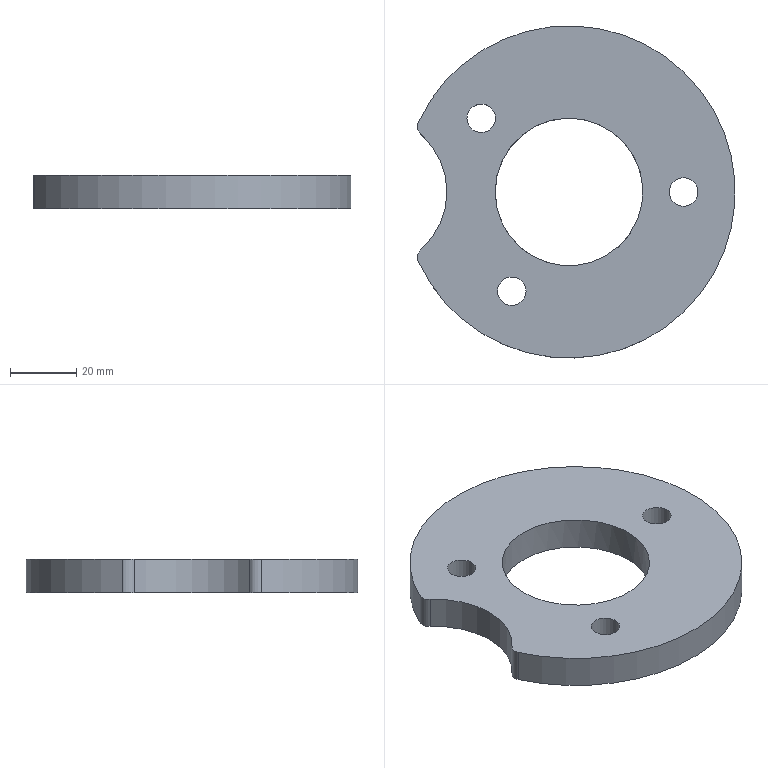Part | STEP file | 1_id1226_x_t | 1 solid | 10 faces | box 95.666 x 100 x 10 mm | volume 57810 mm3 | cylinder 8 | plane 2 | commonest cylinder face diameters 8.6 x3 6 x2 44.45 x1 46.5 x1 100 x1
STEP:
#1=CARTESIAN_POINT('',(0.,0.,0.));
#2=DIRECTION('',(0.,0.,1.));
#3=DIRECTION('',(1.,0.,0.));
#4=AXIS2_PLACEMENT_3D('',#1,#2,#3);
#5=CARTESIAN_POINT('',(817.535,308.471,90.11));
#6=VERTEX_POINT('',#5);
#7=CARTESIAN_POINT('',(817.535,266.529,90.11));
#8=VERTEX_POINT('',#7);
#9=CARTESIAN_POINT('',(862.925,287.5,90.11));
#10=DIRECTION('',(0.,0.,-1.));
#11=DIRECTION('',(1.,0.,0.));
#12=AXIS2_PLACEMENT_3D('',#9,#10,#11);
#13=CIRCLE('',#12,50.);
#14=CARTESIAN_POINT('',(862.925,287.5,90.11));
#15=DIRECTION('',(0.,0.,-1.));
#16=DIRECTION('',(-1.,0.,0.));
#17=AXIS2_PLACEMENT_3D('',#14,#15,#16);
#18=PLANE('',#17);
#19=CARTESIAN_POINT('',(0.,0.));
#20=DIRECTION('',(-1.,0.));
#21=AXIS2_PLACEMENT_2D('',#19,#20);
#22=CIRCLE('',#21,50.);
#23=(GEOMETRIC_REPRESENTATION_CONTEXT(2)PARAMETRIC_REPRESENTATION_CONTEXT()REPRESENTATION_CONTEXT('',''));
#24=DEFINITIONAL_REPRESENTATION('',(#22),#23);
#25=PCURVE('',#18,#24);
#26=CARTESIAN_POINT('',(862.925,287.5,100.11));
#27=DIRECTION('',(0.,0.,-1.));
#28=DIRECTION('',(-1.,0.,0.));
#29=AXIS2_PLACEMENT_3D('',#26,#27,#28);
#30=CYLINDRICAL_SURFACE('',#29,50.);
#31=CARTESIAN_POINT('',(-3.142,10.));
#32=DIRECTION('',(1.,0.));
#33=VECTOR('',#32,1.);
#34=LINE('',#31,#33);
#35=(GEOMETRIC_REPRESENTATION_CONTEXT(2)PARAMETRIC_REPRESENTATION_CONTEXT()REPRESENTATION_CONTEXT('',''));
#36=DEFINITIONAL_REPRESENTATION('',(#34),#35);
#37=PCURVE('',#30,#36);
#38=SURFACE_CURVE('',#13,(#25,#37),.PCURVE_S1.);
#39=EDGE_CURVE('',#6,#8,#38,.T.);
#40=ORIENTED_EDGE('',*,*,#39,.T.);
#41=CARTESIAN_POINT('',(818.278,270.04,90.11));
#42=VERTEX_POINT('',#41);
#43=CARTESIAN_POINT('',(820.259,267.787,90.11));
#44=DIRECTION('',(0.,0.,-1.));
#45=DIRECTION('',(-1.,0.,0.));
#46=AXIS2_PLACEMENT_3D('',#43,#44,#45);
#47=CIRCLE('',#46,3.);
#48=CARTESIAN_POINT('',(42.666,-19.713));
#49=DIRECTION('',(1.,0.));
#50=AXIS2_PLACEMENT_2D('',#48,#49);
#51=CIRCLE('',#50,3.);
#52=(GEOMETRIC_REPRESENTATION_CONTEXT(2)PARAMETRIC_REPRESENTATION_CONTEXT()REPRESENTATION_CONTEXT('',''));
#53=DEFINITIONAL_REPRESENTATION('',(#51),#52);
#54=PCURVE('',#18,#53);
#55=CARTESIAN_POINT('',(820.259,267.787,29.935));
#56=DIRECTION('',(0.,0.,1.));
#57=DIRECTION('',(1.,0.,0.));
#58=AXIS2_PLACEMENT_3D('',#55,#56,#57);
#59=CYLINDRICAL_SURFACE('',#58,3.);
#60=CARTESIAN_POINT('',(9.425,60.175));
#61=DIRECTION('',(-1.,0.));
#62=VECTOR('',#61,1.);
#63=LINE('',#60,#62);
#64=(GEOMETRIC_REPRESENTATION_CONTEXT(2)PARAMETRIC_REPRESENTATION_CONTEXT()REPRESENTATION_CONTEXT('',''));
#65=DEFINITIONAL_REPRESENTATION('',(#63),#64);
#66=PCURVE('',#59,#65);
#67=SURFACE_CURVE('',#47,(#54,#66),.PCURVE_S1.);
#68=EDGE_CURVE('',#8,#42,#67,.T.);
#69=ORIENTED_EDGE('',*,*,#68,.T.);
#70=CARTESIAN_POINT('',(818.278,304.96,90.11));
#71=VERTEX_POINT('',#70);
#72=CARTESIAN_POINT('',(802.925,287.5,90.11));
#73=DIRECTION('',(0.,0.,1.));
#74=DIRECTION('',(1.,0.,0.));
#75=AXIS2_PLACEMENT_3D('',#72,#73,#74);
#76=CIRCLE('',#75,23.25);
#77=CARTESIAN_POINT('',(36.75,0.));
#78=CARTESIAN_POINT('',(36.75,40.27));
#79=CARTESIAN_POINT('',(71.625,20.135));
#80=CARTESIAN_POINT('',(106.5,0.));
#81=CARTESIAN_POINT('',(71.625,-20.135));
#82=CARTESIAN_POINT('',(36.75,-40.27));
#83=CARTESIAN_POINT('',(36.75,0.));
#84=(BOUNDED_CURVE()B_SPLINE_CURVE(2,(#77,#78,#79,#80,#81,#82,#83),.UNSPECIFIED.,.T.,.F.)B_SPLINE_CURVE_WITH_KNOTS((1,2,2,2,2,1),(-2.094,0.,2.094,4.189,6.283,8.378),.UNSPECIFIED.)CURVE()GEOMETRIC_REPRESENTATION_ITEM()RATIONAL_B_SPLINE_CURVE((1.,0.5,1.,0.5,1.,0.5,1.))REPRESENTATION_ITEM(''));
#85=(GEOMETRIC_REPRESENTATION_CONTEXT(2)PARAMETRIC_REPRESENTATION_CONTEXT()REPRESENTATION_CONTEXT('',''));
#86=DEFINITIONAL_REPRESENTATION('',(#84),#85);
#87=PCURVE('',#18,#86);
#88=CARTESIAN_POINT('',(802.925,287.5,29.935));
#89=DIRECTION('',(0.,0.,1.));
#90=DIRECTION('',(1.,0.,0.));
#91=AXIS2_PLACEMENT_3D('',#88,#89,#90);
#92=CYLINDRICAL_SURFACE('',#91,23.25);
#93=CARTESIAN_POINT('',(0.,60.175));
#94=DIRECTION('',(1.,0.));
#95=VECTOR('',#94,1.);
#96=LINE('',#93,#95);
#97=(GEOMETRIC_REPRESENTATION_CONTEXT(2)PARAMETRIC_REPRESENTATION_CONTEXT()REPRESENTATION_CONTEXT('',''));
#98=DEFINITIONAL_REPRESENTATION('',(#96),#97);
#99=PCURVE('',#92,#98);
#100=SURFACE_CURVE('',#76,(#87,#99),.PCURVE_S1.);
#101=EDGE_CURVE('',#42,#71,#100,.T.);
#102=ORIENTED_EDGE('',*,*,#101,.T.);
#103=CARTESIAN_POINT('',(820.259,307.213,90.11));
#104=DIRECTION('',(0.,0.,-1.));
#105=DIRECTION('',(-1.,0.,0.));
#106=AXIS2_PLACEMENT_3D('',#103,#104,#105);
#107=CIRCLE('',#106,3.);
#108=CARTESIAN_POINT('',(42.666,19.713));
#109=DIRECTION('',(1.,0.));
#110=AXIS2_PLACEMENT_2D('',#108,#109);
#111=CIRCLE('',#110,3.);
#112=(GEOMETRIC_REPRESENTATION_CONTEXT(2)PARAMETRIC_REPRESENTATION_CONTEXT()REPRESENTATION_CONTEXT('',''));
#113=DEFINITIONAL_REPRESENTATION('',(#111),#112);
#114=PCURVE('',#18,#113);
#115=CARTESIAN_POINT('',(820.259,307.213,29.935));
#116=DIRECTION('',(0.,0.,-1.));
#117=DIRECTION('',(-1.,0.,0.));
#118=AXIS2_PLACEMENT_3D('',#115,#116,#117);
#119=CYLINDRICAL_SURFACE('',#118,3.);
#120=CARTESIAN_POINT('',(0.,-60.175));
#121=DIRECTION('',(1.,0.));
#122=VECTOR('',#121,1.);
#123=LINE('',#120,#122);
#124=(GEOMETRIC_REPRESENTATION_CONTEXT(2)PARAMETRIC_REPRESENTATION_CONTEXT()REPRESENTATION_CONTEXT('',''));
#125=DEFINITIONAL_REPRESENTATION('',(#123),#124);
#126=PCURVE('',#119,#125);
#127=SURFACE_CURVE('',#107,(#114,#126),.PCURVE_S1.);
#128=EDGE_CURVE('',#71,#6,#127,.T.);
#129=ORIENTED_EDGE('',*,*,#128,.T.);
#130=EDGE_LOOP('',(#40,#69,#102,#129));
#131=FACE_BOUND('',#130,.T.);
#132=CARTESIAN_POINT('',(840.7,287.5,90.11));
#133=VERTEX_POINT('',#132);
#134=CARTESIAN_POINT('',(862.925,287.5,90.11));
#135=DIRECTION('',(0.,0.,1.));
#136=DIRECTION('',(-1.,0.,0.));
#137=AXIS2_PLACEMENT_3D('',#134,#135,#136);
#138=CIRCLE('',#137,22.225);
#139=CARTESIAN_POINT('',(22.225,0.));
#140=CARTESIAN_POINT('',(22.225,-38.495));
#141=CARTESIAN_POINT('',(-11.113,-19.247));
#142=CARTESIAN_POINT('',(-44.45,0.));
#143=CARTESIAN_POINT('',(-11.113,19.247));
#144=CARTESIAN_POINT('',(22.225,38.495));
#145=CARTESIAN_POINT('',(22.225,0.));
#146=(BOUNDED_CURVE()B_SPLINE_CURVE(2,(#139,#140,#141,#142,#143,#144,#145),.UNSPECIFIED.,.T.,.F.)B_SPLINE_CURVE_WITH_KNOTS((1,2,2,2,2,1),(-2.094,0.,2.094,4.189,6.283,8.378),.UNSPECIFIED.)CURVE()GEOMETRIC_REPRESENTATION_ITEM()RATIONAL_B_SPLINE_CURVE((1.,0.5,1.,0.5,1.,0.5,1.))REPRESENTATION_ITEM(''));
#147=(GEOMETRIC_REPRESENTATION_CONTEXT(2)PARAMETRIC_REPRESENTATION_CONTEXT()REPRESENTATION_CONTEXT('',''));
#148=DEFINITIONAL_REPRESENTATION('',(#146),#147);
#149=PCURVE('',#18,#148);
#150=CARTESIAN_POINT('',(862.925,287.5,91.735));
#151=DIRECTION('',(0.,0.,1.));
#152=DIRECTION('',(-0.5,0.866,0.));
#153=AXIS2_PLACEMENT_3D('',#150,#151,#152);
#154=CYLINDRICAL_SURFACE('',#153,22.225);
#155=CARTESIAN_POINT('',(1.047,-1.625));
#156=DIRECTION('',(1.,0.));
#157=VECTOR('',#156,1.);
#158=LINE('',#155,#157);
#159=(GEOMETRIC_REPRESENTATION_CONTEXT(2)PARAMETRIC_REPRESENTATION_CONTEXT()REPRESENTATION_CONTEXT('',''));
#160=DEFINITIONAL_REPRESENTATION('',(#158),#159);
#161=PCURVE('',#154,#160);
#162=SURFACE_CURVE('',#138,(#149,#161),.PCURVE_S1.);
#163=EDGE_CURVE('',#133,#133,#162,.T.);
#164=ORIENTED_EDGE('',*,*,#163,.T.);
#165=EDGE_LOOP('',(#164));
#166=FACE_BOUND('',#165,.T.);
#167=CARTESIAN_POINT('',(849.975,257.622,90.11));
#168=VERTEX_POINT('',#167);
#169=CARTESIAN_POINT('',(845.675,257.622,90.11));
#170=DIRECTION('',(0.,0.,1.));
#171=DIRECTION('',(1.,0.,0.));
#172=AXIS2_PLACEMENT_3D('',#169,#170,#171);
#173=CIRCLE('',#172,4.3);
#174=CARTESIAN_POINT('',(12.95,-29.878));
#175=CARTESIAN_POINT('',(12.95,-22.43));
#176=CARTESIAN_POINT('',(19.4,-26.154));
#177=CARTESIAN_POINT('',(25.85,-29.878));
#178=CARTESIAN_POINT('',(19.4,-33.602));
#179=CARTESIAN_POINT('',(12.95,-37.326));
#180=CARTESIAN_POINT('',(12.95,-29.878));
#181=(BOUNDED_CURVE()B_SPLINE_CURVE(2,(#174,#175,#176,#177,#178,#179,#180),.UNSPECIFIED.,.T.,.F.)B_SPLINE_CURVE_WITH_KNOTS((1,2,2,2,2,1),(-2.094,0.,2.094,4.189,6.283,8.378),.UNSPECIFIED.)CURVE()GEOMETRIC_REPRESENTATION_ITEM()RATIONAL_B_SPLINE_CURVE((1.,0.5,1.,0.5,1.,0.5,1.))REPRESENTATION_ITEM(''));
#182=(GEOMETRIC_REPRESENTATION_CONTEXT(2)PARAMETRIC_REPRESENTATION_CONTEXT()REPRESENTATION_CONTEXT('',''));
#183=DEFINITIONAL_REPRESENTATION('',(#181),#182);
#184=PCURVE('',#18,#183);
#185=CARTESIAN_POINT('',(845.675,257.622,199.11));
#186=DIRECTION('',(0.,0.,-1.));
#187=DIRECTION('',(-1.,0.,0.));
#188=AXIS2_PLACEMENT_3D('',#185,#186,#187);
#189=CYLINDRICAL_SURFACE('',#188,4.3);
#190=CARTESIAN_POINT('',(9.425,109.));
#191=DIRECTION('',(-1.,0.));
#192=VECTOR('',#191,1.);
#193=LINE('',#190,#192);
#194=(GEOMETRIC_REPRESENTATION_CONTEXT(2)PARAMETRIC_REPRESENTATION_CONTEXT()REPRESENTATION_CONTEXT('',''));
#195=DEFINITIONAL_REPRESENTATION('',(#193),#194);
#196=PCURVE('',#189,#195);
#197=SURFACE_CURVE('',#173,(#184,#196),.PCURVE_S1.);
#198=EDGE_CURVE('',#168,#168,#197,.T.);
#199=ORIENTED_EDGE('',*,*,#198,.T.);
#200=EDGE_LOOP('',(#199));
#201=FACE_BOUND('',#200,.T.);
#202=CARTESIAN_POINT('',(901.725,287.5,90.11));
#203=VERTEX_POINT('',#202);
#204=CARTESIAN_POINT('',(897.425,287.5,90.11));
#205=DIRECTION('',(0.,0.,1.));
#206=DIRECTION('',(1.,0.,0.));
#207=AXIS2_PLACEMENT_3D('',#204,#205,#206);
#208=CIRCLE('',#207,4.3);
#209=CARTESIAN_POINT('',(-38.8,0.));
#210=CARTESIAN_POINT('',(-38.8,7.448));
#211=CARTESIAN_POINT('',(-32.35,3.724));
#212=CARTESIAN_POINT('',(-25.9,0.));
#213=CARTESIAN_POINT('',(-32.35,-3.724));
#214=CARTESIAN_POINT('',(-38.8,-7.448));
#215=CARTESIAN_POINT('',(-38.8,0.));
#216=(BOUNDED_CURVE()B_SPLINE_CURVE(2,(#209,#210,#211,#212,#213,#214,#215),.UNSPECIFIED.,.T.,.F.)B_SPLINE_CURVE_WITH_KNOTS((1,2,2,2,2,1),(-2.094,0.,2.094,4.189,6.283,8.378),.UNSPECIFIED.)CURVE()GEOMETRIC_REPRESENTATION_ITEM()RATIONAL_B_SPLINE_CURVE((1.,0.5,1.,0.5,1.,0.5,1.))REPRESENTATION_ITEM(''));
#217=(GEOMETRIC_REPRESENTATION_CONTEXT(2)PARAMETRIC_REPRESENTATION_CONTEXT()REPRESENTATION_CONTEXT('',''));
#218=DEFINITIONAL_REPRESENTATION('',(#216),#217);
#219=PCURVE('',#18,#218);
#220=CARTESIAN_POINT('',(897.425,287.5,199.11));
#221=DIRECTION('',(0.,0.,-1.));
#222=DIRECTION('',(-1.,0.,0.));
#223=AXIS2_PLACEMENT_3D('',#220,#221,#222);
#224=CYLINDRICAL_SURFACE('',#223,4.3);
#225=CARTESIAN_POINT('',(9.425,109.));
#226=DIRECTION('',(-1.,0.));
#227=VECTOR('',#226,1.);
#228=LINE('',#225,#227);
#229=(GEOMETRIC_REPRESENTATION_CONTEXT(2)PARAMETRIC_REPRESENTATION_CONTEXT()REPRESENTATION_CONTEXT('',''));
#230=DEFINITIONAL_REPRESENTATION('',(#228),#229);
#231=PCURVE('',#224,#230);
#232=SURFACE_CURVE('',#208,(#219,#231),.PCURVE_S1.);
#233=EDGE_CURVE('',#203,#203,#232,.T.);
#234=ORIENTED_EDGE('',*,*,#233,.T.);
#235=EDGE_LOOP('',(#234));
#236=FACE_BOUND('',#235,.T.);
#237=CARTESIAN_POINT('',(840.796,309.676,90.11));
#238=VERTEX_POINT('',#237);
#239=CARTESIAN_POINT('',(836.496,309.676,90.11));
#240=DIRECTION('',(0.,0.,1.));
#241=DIRECTION('',(1.,0.,0.));
#242=AXIS2_PLACEMENT_3D('',#239,#240,#241);
#243=CIRCLE('',#242,4.3);
#244=CARTESIAN_POINT('',(22.129,22.176));
#245=CARTESIAN_POINT('',(22.129,29.624));
#246=CARTESIAN_POINT('',(28.579,25.9));
#247=CARTESIAN_POINT('',(35.029,22.176));
#248=CARTESIAN_POINT('',(28.579,18.452));
#249=CARTESIAN_POINT('',(22.129,14.728));
#250=CARTESIAN_POINT('',(22.129,22.176));
#251=(BOUNDED_CURVE()B_SPLINE_CURVE(2,(#244,#245,#246,#247,#248,#249,#250),.UNSPECIFIED.,.T.,.F.)B_SPLINE_CURVE_WITH_KNOTS((1,2,2,2,2,1),(-2.094,0.,2.094,4.189,6.283,8.378),.UNSPECIFIED.)CURVE()GEOMETRIC_REPRESENTATION_ITEM()RATIONAL_B_SPLINE_CURVE((1.,0.5,1.,0.5,1.,0.5,1.))REPRESENTATION_ITEM(''));
#252=(GEOMETRIC_REPRESENTATION_CONTEXT(2)PARAMETRIC_REPRESENTATION_CONTEXT()REPRESENTATION_CONTEXT('',''));
#253=DEFINITIONAL_REPRESENTATION('',(#251),#252);
#254=PCURVE('',#18,#253);
#255=CARTESIAN_POINT('',(836.496,309.676,199.11));
#256=DIRECTION('',(0.,0.,-1.));
#257=DIRECTION('',(-1.,0.,0.));
#258=AXIS2_PLACEMENT_3D('',#255,#256,#257);
#259=CYLINDRICAL_SURFACE('',#258,4.3);
#260=CARTESIAN_POINT('',(9.425,109.));
#261=DIRECTION('',(-1.,0.));
#262=VECTOR('',#261,1.);
#263=LINE('',#260,#262);
#264=(GEOMETRIC_REPRESENTATION_CONTEXT(2)PARAMETRIC_REPRESENTATION_CONTEXT()REPRESENTATION_CONTEXT('',''));
#265=DEFINITIONAL_REPRESENTATION('',(#263),#264);
#266=PCURVE('',#259,#265);
#267=SURFACE_CURVE('',#243,(#254,#266),.PCURVE_S1.);
#268=EDGE_CURVE('',#238,#238,#267,.T.);
#269=ORIENTED_EDGE('',*,*,#268,.T.);
#270=EDGE_LOOP('',(#269));
#271=FACE_BOUND('',#270,.T.);
#272=ADVANCED_FACE('',(#131,#166,#201,#236,#271),#18,.T.);
#273=CARTESIAN_POINT('',(874.038,268.253,100.11));
#274=VERTEX_POINT('',#273);
#275=CARTESIAN_POINT('',(840.7,287.5,100.11));
#276=VERTEX_POINT('',#275);
#277=CARTESIAN_POINT('',(862.925,287.5,100.11));
#278=DIRECTION('',(0.,0.,-1.));
#279=DIRECTION('',(0.5,-0.866,0.));
#280=AXIS2_PLACEMENT_3D('',#277,#278,#279);
#281=CIRCLE('',#280,22.225);
#282=CARTESIAN_POINT('',(3.142,8.375));
#283=DIRECTION('',(-1.,0.));
#284=VECTOR('',#283,1.);
#285=LINE('',#282,#284);
#286=(GEOMETRIC_REPRESENTATION_CONTEXT(2)PARAMETRIC_REPRESENTATION_CONTEXT()REPRESENTATION_CONTEXT('',''));
#287=DEFINITIONAL_REPRESENTATION('',(#285),#286);
#288=PCURVE('',#154,#287);
#289=CARTESIAN_POINT('',(862.925,287.5,100.11));
#290=DIRECTION('',(0.,0.,-1.));
#291=DIRECTION('',(-1.,0.,0.));
#292=AXIS2_PLACEMENT_3D('',#289,#290,#291);
#293=PLANE('',#292);
#294=CARTESIAN_POINT('',(0.,0.));
#295=DIRECTION('',(-0.5,-0.866));
#296=AXIS2_PLACEMENT_2D('',#294,#295);
#297=CIRCLE('',#296,22.225);
#298=(GEOMETRIC_REPRESENTATION_CONTEXT(2)PARAMETRIC_REPRESENTATION_CONTEXT()REPRESENTATION_CONTEXT('',''));
#299=DEFINITIONAL_REPRESENTATION('',(#297),#298);
#300=PCURVE('',#293,#299);
#301=SURFACE_CURVE('',#281,(#288,#300),.PCURVE_S1.);
#302=EDGE_CURVE('',#274,#276,#301,.T.);
#303=ORIENTED_EDGE('',*,*,#302,.T.);
#304=CARTESIAN_POINT('',(840.7,287.5,90.11));
#305=CARTESIAN_POINT('',(840.7,287.5,100.11));
#306=B_SPLINE_CURVE_WITH_KNOTS('',1,(#304,#305),.UNSPECIFIED.,.F.,.F.,(2,2),(-1.625,8.375),.PIECEWISE_BEZIER_KNOTS.);
#307=CARTESIAN_POINT('',(1.047,0.));
#308=DIRECTION('',(0.,1.));
#309=VECTOR('',#308,1.);
#310=LINE('',#307,#309);
#311=(GEOMETRIC_REPRESENTATION_CONTEXT(2)PARAMETRIC_REPRESENTATION_CONTEXT()REPRESENTATION_CONTEXT('',''));
#312=DEFINITIONAL_REPRESENTATION('',(#310),#311);
#313=PCURVE('',#154,#312);
#314=CARTESIAN_POINT('',(7.33,0.));
#315=DIRECTION('',(0.,1.));
#316=VECTOR('',#315,1.);
#317=LINE('',#314,#316);
#318=(GEOMETRIC_REPRESENTATION_CONTEXT(2)PARAMETRIC_REPRESENTATION_CONTEXT()REPRESENTATION_CONTEXT('',''));
#319=DEFINITIONAL_REPRESENTATION('',(#317),#318);
#320=PCURVE('',#154,#319);
#321=SEAM_CURVE('',#306,(#313,#320),.PCURVE_S1.);
#322=EDGE_CURVE('',#133,#276,#321,.T.);
#323=ORIENTED_EDGE('',*,*,#322,.F.);
#324=ORIENTED_EDGE('',*,*,#163,.T.);
#325=ORIENTED_EDGE('',*,*,#322,.T.);
#326=CARTESIAN_POINT('',(862.925,287.5,100.11));
#327=DIRECTION('',(0.,0.,-1.));
#328=DIRECTION('',(0.5,-0.866,0.));
#329=AXIS2_PLACEMENT_3D('',#326,#327,#328);
#330=CIRCLE('',#329,22.225);
#331=CARTESIAN_POINT('',(9.425,8.375));
#332=DIRECTION('',(-1.,0.));
#333=VECTOR('',#332,1.);
#334=LINE('',#331,#333);
#335=(GEOMETRIC_REPRESENTATION_CONTEXT(2)PARAMETRIC_REPRESENTATION_CONTEXT()REPRESENTATION_CONTEXT('',''));
#336=DEFINITIONAL_REPRESENTATION('',(#334),#335);
#337=PCURVE('',#154,#336);
#338=CARTESIAN_POINT('',(0.,0.));
#339=DIRECTION('',(-0.5,-0.866));
#340=AXIS2_PLACEMENT_2D('',#338,#339);
#341=CIRCLE('',#340,22.225);
#342=(GEOMETRIC_REPRESENTATION_CONTEXT(2)PARAMETRIC_REPRESENTATION_CONTEXT()REPRESENTATION_CONTEXT('',''));
#343=DEFINITIONAL_REPRESENTATION('',(#341),#342);
#344=PCURVE('',#293,#343);
#345=SURFACE_CURVE('',#330,(#337,#344),.PCURVE_S1.);
#346=EDGE_CURVE('',#276,#274,#345,.T.);
#347=ORIENTED_EDGE('',*,*,#346,.T.);
#348=EDGE_LOOP('',(#303,#323,#324,#325,#347));
#349=FACE_BOUND('',#348,.F.);
#350=ADVANCED_FACE('',(#349),#154,.F.);
#351=CARTESIAN_POINT('',(818.278,304.96,100.11));
#352=VERTEX_POINT('',#351);
#353=CARTESIAN_POINT('',(818.278,270.04,100.11));
#354=VERTEX_POINT('',#353);
#355=CARTESIAN_POINT('',(802.925,287.5,100.11));
#356=DIRECTION('',(0.,0.,-1.));
#357=DIRECTION('',(1.,0.,0.));
#358=AXIS2_PLACEMENT_3D('',#355,#356,#357);
#359=CIRCLE('',#358,23.25);
#360=CARTESIAN_POINT('',(60.,0.));
#361=DIRECTION('',(-1.,0.));
#362=AXIS2_PLACEMENT_2D('',#360,#361);
#363=CIRCLE('',#362,23.25);
#364=(GEOMETRIC_REPRESENTATION_CONTEXT(2)PARAMETRIC_REPRESENTATION_CONTEXT()REPRESENTATION_CONTEXT('',''));
#365=DEFINITIONAL_REPRESENTATION('',(#363),#364);
#366=PCURVE('',#293,#365);
#367=CARTESIAN_POINT('',(12.566,70.175));
#368=DIRECTION('',(-1.,0.));
#369=VECTOR('',#368,1.);
#370=LINE('',#367,#369);
#371=(GEOMETRIC_REPRESENTATION_CONTEXT(2)PARAMETRIC_REPRESENTATION_CONTEXT()REPRESENTATION_CONTEXT('',''));
#372=DEFINITIONAL_REPRESENTATION('',(#370),#371);
#373=PCURVE('',#92,#372);
#374=SURFACE_CURVE('',#359,(#366,#373),.PCURVE_S1.);
#375=EDGE_CURVE('',#352,#354,#374,.T.);
#376=ORIENTED_EDGE('',*,*,#375,.T.);
#377=CARTESIAN_POINT('',(817.535,266.529,100.11));
#378=VERTEX_POINT('',#377);
#379=CARTESIAN_POINT('',(820.259,267.787,100.11));
#380=DIRECTION('',(0.,0.,1.));
#381=DIRECTION('',(-1.,0.,0.));
#382=AXIS2_PLACEMENT_3D('',#379,#380,#381);
#383=CIRCLE('',#382,3.);
#384=CARTESIAN_POINT('',(45.666,-19.713));
#385=CARTESIAN_POINT('',(45.666,-24.909));
#386=CARTESIAN_POINT('',(41.166,-22.311));
#387=CARTESIAN_POINT('',(36.666,-19.713));
#388=CARTESIAN_POINT('',(41.166,-17.115));
#389=CARTESIAN_POINT('',(45.666,-14.517));
#390=CARTESIAN_POINT('',(45.666,-19.713));
#391=(BOUNDED_CURVE()B_SPLINE_CURVE(2,(#384,#385,#386,#387,#388,#389,#390),.UNSPECIFIED.,.T.,.F.)B_SPLINE_CURVE_WITH_KNOTS((1,2,2,2,2,1),(-2.094,0.,2.094,4.189,6.283,8.378),.UNSPECIFIED.)CURVE()GEOMETRIC_REPRESENTATION_ITEM()RATIONAL_B_SPLINE_CURVE((1.,0.5,1.,0.5,1.,0.5,1.))REPRESENTATION_ITEM(''));
#392=(GEOMETRIC_REPRESENTATION_CONTEXT(2)PARAMETRIC_REPRESENTATION_CONTEXT()REPRESENTATION_CONTEXT('',''));
#393=DEFINITIONAL_REPRESENTATION('',(#391),#392);
#394=PCURVE('',#293,#393);
#395=CARTESIAN_POINT('',(-3.142,70.175));
#396=DIRECTION('',(1.,0.));
#397=VECTOR('',#396,1.);
#398=LINE('',#395,#397);
#399=(GEOMETRIC_REPRESENTATION_CONTEXT(2)PARAMETRIC_REPRESENTATION_CONTEXT()REPRESENTATION_CONTEXT('',''));
#400=DEFINITIONAL_REPRESENTATION('',(#398),#399);
#401=PCURVE('',#59,#400);
#402=SURFACE_CURVE('',#383,(#394,#401),.PCURVE_S1.);
#403=EDGE_CURVE('',#354,#378,#402,.T.);
#404=ORIENTED_EDGE('',*,*,#403,.T.);
#405=CARTESIAN_POINT('',(817.535,308.471,100.11));
#406=VERTEX_POINT('',#405);
#407=CARTESIAN_POINT('',(862.925,287.5,100.11));
#408=DIRECTION('',(0.,0.,1.));
#409=DIRECTION('',(1.,0.,0.));
#410=AXIS2_PLACEMENT_3D('',#407,#408,#409);
#411=CIRCLE('',#410,50.);
#412=CARTESIAN_POINT('',(-50.,0.000000002));
#413=CARTESIAN_POINT('',(-50.,86.603));
#414=CARTESIAN_POINT('',(25.,43.301));
#415=CARTESIAN_POINT('',(100.,-0.000000003));
#416=CARTESIAN_POINT('',(25.,-43.301));
#417=CARTESIAN_POINT('',(-50.,-86.603));
#418=CARTESIAN_POINT('',(-50.,0.000000002));
#419=(BOUNDED_CURVE()B_SPLINE_CURVE(2,(#412,#413,#414,#415,#416,#417,#418),.UNSPECIFIED.,.T.,.F.)B_SPLINE_CURVE_WITH_KNOTS((1,2,2,2,2,1),(-2.094,0.,2.094,4.189,6.283,8.378),.UNSPECIFIED.)CURVE()GEOMETRIC_REPRESENTATION_ITEM()RATIONAL_B_SPLINE_CURVE((1.,0.5,1.,0.5,1.,0.5,1.))REPRESENTATION_ITEM(''));
#420=(GEOMETRIC_REPRESENTATION_CONTEXT(2)PARAMETRIC_REPRESENTATION_CONTEXT()REPRESENTATION_CONTEXT('',''));
#421=DEFINITIONAL_REPRESENTATION('',(#419),#420);
#422=PCURVE('',#293,#421);
#423=CARTESIAN_POINT('',(9.425,0.));
#424=DIRECTION('',(-1.,0.));
#425=VECTOR('',#424,1.);
#426=LINE('',#423,#425);
#427=(GEOMETRIC_REPRESENTATION_CONTEXT(2)PARAMETRIC_REPRESENTATION_CONTEXT()REPRESENTATION_CONTEXT('',''));
#428=DEFINITIONAL_REPRESENTATION('',(#426),#427);
#429=PCURVE('',#30,#428);
#430=SURFACE_CURVE('',#411,(#422,#429),.PCURVE_S1.);
#431=EDGE_CURVE('',#378,#406,#430,.T.);
#432=ORIENTED_EDGE('',*,*,#431,.T.);
#433=CARTESIAN_POINT('',(820.259,307.213,100.11));
#434=DIRECTION('',(0.,0.,1.));
#435=DIRECTION('',(-1.,0.,0.));
#436=AXIS2_PLACEMENT_3D('',#433,#434,#435);
#437=CIRCLE('',#436,3.);
#438=CARTESIAN_POINT('',(45.666,19.713));
#439=CARTESIAN_POINT('',(45.666,14.517));
#440=CARTESIAN_POINT('',(41.166,17.115));
#441=CARTESIAN_POINT('',(36.666,19.713));
#442=CARTESIAN_POINT('',(41.166,22.311));
#443=CARTESIAN_POINT('',(45.666,24.909));
#444=CARTESIAN_POINT('',(45.666,19.713));
#445=(BOUNDED_CURVE()B_SPLINE_CURVE(2,(#438,#439,#440,#441,#442,#443,#444),.UNSPECIFIED.,.T.,.F.)B_SPLINE_CURVE_WITH_KNOTS((1,2,2,2,2,1),(-2.094,0.,2.094,4.189,6.283,8.378),.UNSPECIFIED.)CURVE()GEOMETRIC_REPRESENTATION_ITEM()RATIONAL_B_SPLINE_CURVE((1.,0.5,1.,0.5,1.,0.5,1.))REPRESENTATION_ITEM(''));
#446=(GEOMETRIC_REPRESENTATION_CONTEXT(2)PARAMETRIC_REPRESENTATION_CONTEXT()REPRESENTATION_CONTEXT('',''));
#447=DEFINITIONAL_REPRESENTATION('',(#445),#446);
#448=PCURVE('',#293,#447);
#449=CARTESIAN_POINT('',(12.566,-70.175));
#450=DIRECTION('',(-1.,0.));
#451=VECTOR('',#450,1.);
#452=LINE('',#449,#451);
#453=(GEOMETRIC_REPRESENTATION_CONTEXT(2)PARAMETRIC_REPRESENTATION_CONTEXT()REPRESENTATION_CONTEXT('',''));
#454=DEFINITIONAL_REPRESENTATION('',(#452),#453);
#455=PCURVE('',#119,#454);
#456=SURFACE_CURVE('',#437,(#448,#455),.PCURVE_S1.);
#457=EDGE_CURVE('',#406,#352,#456,.T.);
#458=ORIENTED_EDGE('',*,*,#457,.T.);
#459=EDGE_LOOP('',(#376,#404,#432,#458));
#460=FACE_BOUND('',#459,.T.);
#461=ORIENTED_EDGE('',*,*,#302,.T.);
#462=ORIENTED_EDGE('',*,*,#346,.T.);
#463=EDGE_LOOP('',(#461,#462));
#464=FACE_BOUND('',#463,.T.);
#465=CARTESIAN_POINT('',(849.975,257.622,100.11));
#466=VERTEX_POINT('',#465);
#467=CARTESIAN_POINT('',(845.675,257.622,100.11));
#468=DIRECTION('',(0.,0.,-1.));
#469=DIRECTION('',(1.,0.,0.));
#470=AXIS2_PLACEMENT_3D('',#467,#468,#469);
#471=CIRCLE('',#470,4.3);
#472=CARTESIAN_POINT('',(17.25,-29.878));
#473=DIRECTION('',(-1.,0.));
#474=AXIS2_PLACEMENT_2D('',#472,#473);
#475=CIRCLE('',#474,4.3);
#476=(GEOMETRIC_REPRESENTATION_CONTEXT(2)PARAMETRIC_REPRESENTATION_CONTEXT()REPRESENTATION_CONTEXT('',''));
#477=DEFINITIONAL_REPRESENTATION('',(#475),#476);
#478=PCURVE('',#293,#477);
#479=CARTESIAN_POINT('',(3.142,99.));
#480=DIRECTION('',(1.,0.));
#481=VECTOR('',#480,1.);
#482=LINE('',#479,#481);
#483=(GEOMETRIC_REPRESENTATION_CONTEXT(2)PARAMETRIC_REPRESENTATION_CONTEXT()REPRESENTATION_CONTEXT('',''));
#484=DEFINITIONAL_REPRESENTATION('',(#482),#483);
#485=PCURVE('',#189,#484);
#486=SURFACE_CURVE('',#471,(#478,#485),.PCURVE_S1.);
#487=EDGE_CURVE('',#466,#466,#486,.T.);
#488=ORIENTED_EDGE('',*,*,#487,.T.);
#489=EDGE_LOOP('',(#488));
#490=FACE_BOUND('',#489,.T.);
#491=CARTESIAN_POINT('',(901.725,287.5,100.11));
#492=VERTEX_POINT('',#491);
#493=CARTESIAN_POINT('',(897.425,287.5,100.11));
#494=DIRECTION('',(0.,0.,-1.));
#495=DIRECTION('',(1.,0.,0.));
#496=AXIS2_PLACEMENT_3D('',#493,#494,#495);
#497=CIRCLE('',#496,4.3);
#498=CARTESIAN_POINT('',(-34.5,0.));
#499=DIRECTION('',(-1.,0.));
#500=AXIS2_PLACEMENT_2D('',#498,#499);
#501=CIRCLE('',#500,4.3);
#502=(GEOMETRIC_REPRESENTATION_CONTEXT(2)PARAMETRIC_REPRESENTATION_CONTEXT()REPRESENTATION_CONTEXT('',''));
#503=DEFINITIONAL_REPRESENTATION('',(#501),#502);
#504=PCURVE('',#293,#503);
#505=CARTESIAN_POINT('',(3.142,99.));
#506=DIRECTION('',(1.,0.));
#507=VECTOR('',#506,1.);
#508=LINE('',#505,#507);
#509=(GEOMETRIC_REPRESENTATION_CONTEXT(2)PARAMETRIC_REPRESENTATION_CONTEXT()REPRESENTATION_CONTEXT('',''));
#510=DEFINITIONAL_REPRESENTATION('',(#508),#509);
#511=PCURVE('',#224,#510);
#512=SURFACE_CURVE('',#497,(#504,#511),.PCURVE_S1.);
#513=EDGE_CURVE('',#492,#492,#512,.T.);
#514=ORIENTED_EDGE('',*,*,#513,.T.);
#515=EDGE_LOOP('',(#514));
#516=FACE_BOUND('',#515,.T.);
#517=CARTESIAN_POINT('',(840.796,309.676,100.11));
#518=VERTEX_POINT('',#517);
#519=CARTESIAN_POINT('',(836.496,309.676,100.11));
#520=DIRECTION('',(0.,0.,-1.));
#521=DIRECTION('',(1.,0.,0.));
#522=AXIS2_PLACEMENT_3D('',#519,#520,#521);
#523=CIRCLE('',#522,4.3);
#524=CARTESIAN_POINT('',(26.429,22.176));
#525=DIRECTION('',(-1.,0.));
#526=AXIS2_PLACEMENT_2D('',#524,#525);
#527=CIRCLE('',#526,4.3);
#528=(GEOMETRIC_REPRESENTATION_CONTEXT(2)PARAMETRIC_REPRESENTATION_CONTEXT()REPRESENTATION_CONTEXT('',''));
#529=DEFINITIONAL_REPRESENTATION('',(#527),#528);
#530=PCURVE('',#293,#529);
#531=CARTESIAN_POINT('',(3.142,99.));
#532=DIRECTION('',(1.,0.));
#533=VECTOR('',#532,1.);
#534=LINE('',#531,#533);
#535=(GEOMETRIC_REPRESENTATION_CONTEXT(2)PARAMETRIC_REPRESENTATION_CONTEXT()REPRESENTATION_CONTEXT('',''));
#536=DEFINITIONAL_REPRESENTATION('',(#534),#535);
#537=PCURVE('',#259,#536);
#538=SURFACE_CURVE('',#523,(#530,#537),.PCURVE_S1.);
#539=EDGE_CURVE('',#518,#518,#538,.T.);
#540=ORIENTED_EDGE('',*,*,#539,.T.);
#541=EDGE_LOOP('',(#540));
#542=FACE_BOUND('',#541,.T.);
#543=ADVANCED_FACE('',(#460,#464,#490,#516,#542),#293,.F.);
#544=ORIENTED_EDGE('',*,*,#198,.T.);
#545=CARTESIAN_POINT('',(849.975,257.622,100.11));
#546=CARTESIAN_POINT('',(849.975,257.622,90.11));
#547=B_SPLINE_CURVE_WITH_KNOTS('',1,(#545,#546),.UNSPECIFIED.,.F.,.F.,(2,2),(99.,109.),.PIECEWISE_BEZIER_KNOTS.);
#548=CARTESIAN_POINT('',(3.142,0.));
#549=DIRECTION('',(0.,1.));
#550=VECTOR('',#549,1.);
#551=LINE('',#548,#550);
#552=(GEOMETRIC_REPRESENTATION_CONTEXT(2)PARAMETRIC_REPRESENTATION_CONTEXT()REPRESENTATION_CONTEXT('',''));
#553=DEFINITIONAL_REPRESENTATION('',(#551),#552);
#554=PCURVE('',#189,#553);
#555=CARTESIAN_POINT('',(9.425,0.));
#556=DIRECTION('',(0.,1.));
#557=VECTOR('',#556,1.);
#558=LINE('',#555,#557);
#559=(GEOMETRIC_REPRESENTATION_CONTEXT(2)PARAMETRIC_REPRESENTATION_CONTEXT()REPRESENTATION_CONTEXT('',''));
#560=DEFINITIONAL_REPRESENTATION('',(#558),#559);
#561=PCURVE('',#189,#560);
#562=SEAM_CURVE('',#547,(#554,#561),.PCURVE_S1.);
#563=EDGE_CURVE('',#466,#168,#562,.T.);
#564=ORIENTED_EDGE('',*,*,#563,.F.);
#565=ORIENTED_EDGE('',*,*,#487,.T.);
#566=ORIENTED_EDGE('',*,*,#563,.T.);
#567=EDGE_LOOP('',(#544,#564,#565,#566));
#568=FACE_BOUND('',#567,.F.);
#569=ADVANCED_FACE('',(#568),#189,.F.);
#570=CARTESIAN_POINT('',(818.278,270.04,100.11));
#571=DIRECTION('',(0.,0.,-1.));
#572=VECTOR('',#571,1.);
#573=LINE('',#570,#572);
#574=CARTESIAN_POINT('',(5.434,70.175));
#575=DIRECTION('',(0.,-1.));
#576=VECTOR('',#575,1.);
#577=LINE('',#574,#576);
#578=(GEOMETRIC_REPRESENTATION_CONTEXT(2)PARAMETRIC_REPRESENTATION_CONTEXT()REPRESENTATION_CONTEXT('',''));
#579=DEFINITIONAL_REPRESENTATION('',(#577),#578);
#580=PCURVE('',#92,#579);
#581=CARTESIAN_POINT('',(2.292,70.175));
#582=DIRECTION('',(0.,-1.));
#583=VECTOR('',#582,1.);
#584=LINE('',#581,#583);
#585=(GEOMETRIC_REPRESENTATION_CONTEXT(2)PARAMETRIC_REPRESENTATION_CONTEXT()REPRESENTATION_CONTEXT('',''));
#586=DEFINITIONAL_REPRESENTATION('',(#584),#585);
#587=PCURVE('',#59,#586);
#588=SURFACE_CURVE('',#573,(#580,#587),.PCURVE_S1.);
#589=EDGE_CURVE('',#354,#42,#588,.T.);
#590=ORIENTED_EDGE('',*,*,#589,.T.);
#591=ORIENTED_EDGE('',*,*,#101,.T.);
#592=CARTESIAN_POINT('',(818.278,304.96,90.11));
#593=DIRECTION('',(0.,0.,1.));
#594=VECTOR('',#593,1.);
#595=LINE('',#592,#594);
#596=CARTESIAN_POINT('',(7.133,60.175));
#597=DIRECTION('',(0.,1.));
#598=VECTOR('',#597,1.);
#599=LINE('',#596,#598);
#600=(GEOMETRIC_REPRESENTATION_CONTEXT(2)PARAMETRIC_REPRESENTATION_CONTEXT()REPRESENTATION_CONTEXT('',''));
#601=DEFINITIONAL_REPRESENTATION('',(#599),#600);
#602=PCURVE('',#92,#601);
#603=CARTESIAN_POINT('',(5.434,-60.175));
#604=DIRECTION('',(0.,-1.));
#605=VECTOR('',#604,1.);
#606=LINE('',#603,#605);
#607=(GEOMETRIC_REPRESENTATION_CONTEXT(2)PARAMETRIC_REPRESENTATION_CONTEXT()REPRESENTATION_CONTEXT('',''));
#608=DEFINITIONAL_REPRESENTATION('',(#606),#607);
#609=PCURVE('',#119,#608);
#610=SURFACE_CURVE('',#595,(#602,#609),.PCURVE_S1.);
#611=EDGE_CURVE('',#71,#352,#610,.T.);
#612=ORIENTED_EDGE('',*,*,#611,.T.);
#613=ORIENTED_EDGE('',*,*,#375,.T.);
#614=EDGE_LOOP('',(#590,#591,#612,#613));
#615=FACE_BOUND('',#614,.F.);
#616=ADVANCED_FACE('',(#615),#92,.F.);
#617=ORIENTED_EDGE('',*,*,#403,.F.);
#618=ORIENTED_EDGE('',*,*,#589,.T.);
#619=ORIENTED_EDGE('',*,*,#68,.F.);
#620=CARTESIAN_POINT('',(817.535,266.529,90.11));
#621=DIRECTION('',(0.,0.,1.));
#622=VECTOR('',#621,1.);
#623=LINE('',#620,#622);
#624=CARTESIAN_POINT('',(3.574,60.175));
#625=DIRECTION('',(0.,1.));
#626=VECTOR('',#625,1.);
#627=LINE('',#624,#626);
#628=(GEOMETRIC_REPRESENTATION_CONTEXT(2)PARAMETRIC_REPRESENTATION_CONTEXT()REPRESENTATION_CONTEXT('',''));
#629=DEFINITIONAL_REPRESENTATION('',(#627),#628);
#630=PCURVE('',#59,#629);
#631=CARTESIAN_POINT('',(5.85,10.));
#632=DIRECTION('',(0.,-1.));
#633=VECTOR('',#632,1.);
#634=LINE('',#631,#633);
#635=(GEOMETRIC_REPRESENTATION_CONTEXT(2)PARAMETRIC_REPRESENTATION_CONTEXT()REPRESENTATION_CONTEXT('',''));
#636=DEFINITIONAL_REPRESENTATION('',(#634),#635);
#637=PCURVE('',#30,#636);
#638=SURFACE_CURVE('',#623,(#630,#637),.PCURVE_S1.);
#639=EDGE_CURVE('',#8,#378,#638,.T.);
#640=ORIENTED_EDGE('',*,*,#639,.T.);
#641=EDGE_LOOP('',(#617,#618,#619,#640));
#642=FACE_BOUND('',#641,.T.);
#643=ADVANCED_FACE('',(#642),#59,.T.);
#644=ORIENTED_EDGE('',*,*,#39,.F.);
#645=CARTESIAN_POINT('',(817.535,308.471,100.11));
#646=DIRECTION('',(0.,0.,-1.));
#647=VECTOR('',#646,1.);
#648=LINE('',#645,#647);
#649=CARTESIAN_POINT('',(0.4328,0.));
#650=DIRECTION('',(0.,1.));
#651=VECTOR('',#650,1.);
#652=LINE('',#649,#651);
#653=(GEOMETRIC_REPRESENTATION_CONTEXT(2)PARAMETRIC_REPRESENTATION_CONTEXT()REPRESENTATION_CONTEXT('',''));
#654=DEFINITIONAL_REPRESENTATION('',(#652),#653);
#655=PCURVE('',#30,#654);
#656=CARTESIAN_POINT('',(6.716,-70.175));
#657=DIRECTION('',(0.,1.));
#658=VECTOR('',#657,1.);
#659=LINE('',#656,#658);
#660=(GEOMETRIC_REPRESENTATION_CONTEXT(2)PARAMETRIC_REPRESENTATION_CONTEXT()REPRESENTATION_CONTEXT('',''));
#661=DEFINITIONAL_REPRESENTATION('',(#659),#660);
#662=PCURVE('',#119,#661);
#663=SURFACE_CURVE('',#648,(#655,#662),.PCURVE_S1.);
#664=EDGE_CURVE('',#406,#6,#663,.T.);
#665=ORIENTED_EDGE('',*,*,#664,.F.);
#666=ORIENTED_EDGE('',*,*,#431,.F.);
#667=ORIENTED_EDGE('',*,*,#639,.F.);
#668=EDGE_LOOP('',(#644,#665,#666,#667));
#669=FACE_BOUND('',#668,.T.);
#670=ADVANCED_FACE('',(#669),#30,.T.);
#671=ORIENTED_EDGE('',*,*,#128,.F.);
#672=ORIENTED_EDGE('',*,*,#611,.T.);
#673=ORIENTED_EDGE('',*,*,#457,.F.);
#674=ORIENTED_EDGE('',*,*,#664,.T.);
#675=EDGE_LOOP('',(#671,#672,#673,#674));
#676=FACE_BOUND('',#675,.T.);
#677=ADVANCED_FACE('',(#676),#119,.T.);
#678=ORIENTED_EDGE('',*,*,#233,.T.);
#679=CARTESIAN_POINT('',(901.725,287.5,100.11));
#680=CARTESIAN_POINT('',(901.725,287.5,90.11));
#681=B_SPLINE_CURVE_WITH_KNOTS('',1,(#679,#680),.UNSPECIFIED.,.F.,.F.,(2,2),(99.,109.),.PIECEWISE_BEZIER_KNOTS.);
#682=CARTESIAN_POINT('',(3.142,0.));
#683=DIRECTION('',(0.,1.));
#684=VECTOR('',#683,1.);
#685=LINE('',#682,#684);
#686=(GEOMETRIC_REPRESENTATION_CONTEXT(2)PARAMETRIC_REPRESENTATION_CONTEXT()REPRESENTATION_CONTEXT('',''));
#687=DEFINITIONAL_REPRESENTATION('',(#685),#686);
#688=PCURVE('',#224,#687);
#689=CARTESIAN_POINT('',(9.425,0.));
#690=DIRECTION('',(0.,1.));
#691=VECTOR('',#690,1.);
#692=LINE('',#689,#691);
#693=(GEOMETRIC_REPRESENTATION_CONTEXT(2)PARAMETRIC_REPRESENTATION_CONTEXT()REPRESENTATION_CONTEXT('',''));
#694=DEFINITIONAL_REPRESENTATION('',(#692),#693);
#695=PCURVE('',#224,#694);
#696=SEAM_CURVE('',#681,(#688,#695),.PCURVE_S1.);
#697=EDGE_CURVE('',#492,#203,#696,.T.);
#698=ORIENTED_EDGE('',*,*,#697,.F.);
#699=ORIENTED_EDGE('',*,*,#513,.T.);
#700=ORIENTED_EDGE('',*,*,#697,.T.);
#701=EDGE_LOOP('',(#678,#698,#699,#700));
#702=FACE_BOUND('',#701,.F.);
#703=ADVANCED_FACE('',(#702),#224,.F.);
#704=ORIENTED_EDGE('',*,*,#268,.T.);
#705=CARTESIAN_POINT('',(840.796,309.676,100.11));
#706=CARTESIAN_POINT('',(840.796,309.676,90.11));
#707=B_SPLINE_CURVE_WITH_KNOTS('',1,(#705,#706),.UNSPECIFIED.,.F.,.F.,(2,2),(99.,109.),.PIECEWISE_BEZIER_KNOTS.);
#708=CARTESIAN_POINT('',(3.142,0.));
#709=DIRECTION('',(0.,1.));
#710=VECTOR('',#709,1.);
#711=LINE('',#708,#710);
#712=(GEOMETRIC_REPRESENTATION_CONTEXT(2)PARAMETRIC_REPRESENTATION_CONTEXT()REPRESENTATION_CONTEXT('',''));
#713=DEFINITIONAL_REPRESENTATION('',(#711),#712);
#714=PCURVE('',#259,#713);
#715=CARTESIAN_POINT('',(9.425,0.));
#716=DIRECTION('',(0.,1.));
#717=VECTOR('',#716,1.);
#718=LINE('',#715,#717);
#719=(GEOMETRIC_REPRESENTATION_CONTEXT(2)PARAMETRIC_REPRESENTATION_CONTEXT()REPRESENTATION_CONTEXT('',''));
#720=DEFINITIONAL_REPRESENTATION('',(#718),#719);
#721=PCURVE('',#259,#720);
#722=SEAM_CURVE('',#707,(#714,#721),.PCURVE_S1.);
#723=EDGE_CURVE('',#518,#238,#722,.T.);
#724=ORIENTED_EDGE('',*,*,#723,.F.);
#725=ORIENTED_EDGE('',*,*,#539,.T.);
#726=ORIENTED_EDGE('',*,*,#723,.T.);
#727=EDGE_LOOP('',(#704,#724,#725,#726));
#728=FACE_BOUND('',#727,.F.);
#729=ADVANCED_FACE('',(#728),#259,.F.);
#730=CLOSED_SHELL('',(#272,#350,#543,#569,#616,#643,#670,#677,#703,#729));
#731=MANIFOLD_SOLID_BREP('',#730);
#732=(LENGTH_UNIT()NAMED_UNIT(*)SI_UNIT(.MILLI.,.METRE.));
#733=UNCERTAINTY_MEASURE_WITH_UNIT(LENGTH_MEASURE(0.000005),#732,'','');
#734=(NAMED_UNIT(*)PLANE_ANGLE_UNIT()SI_UNIT($,.RADIAN.));
#735=(NAMED_UNIT(*)SI_UNIT($,.STERADIAN.)SOLID_ANGLE_UNIT());
#736=(GEOMETRIC_REPRESENTATION_CONTEXT(3)GLOBAL_UNCERTAINTY_ASSIGNED_CONTEXT((#733))GLOBAL_UNIT_ASSIGNED_CONTEXT((#732,#734,#735))REPRESENTATION_CONTEXT('',''));
#737=ADVANCED_BREP_SHAPE_REPRESENTATION('',(#4,#731),#736);